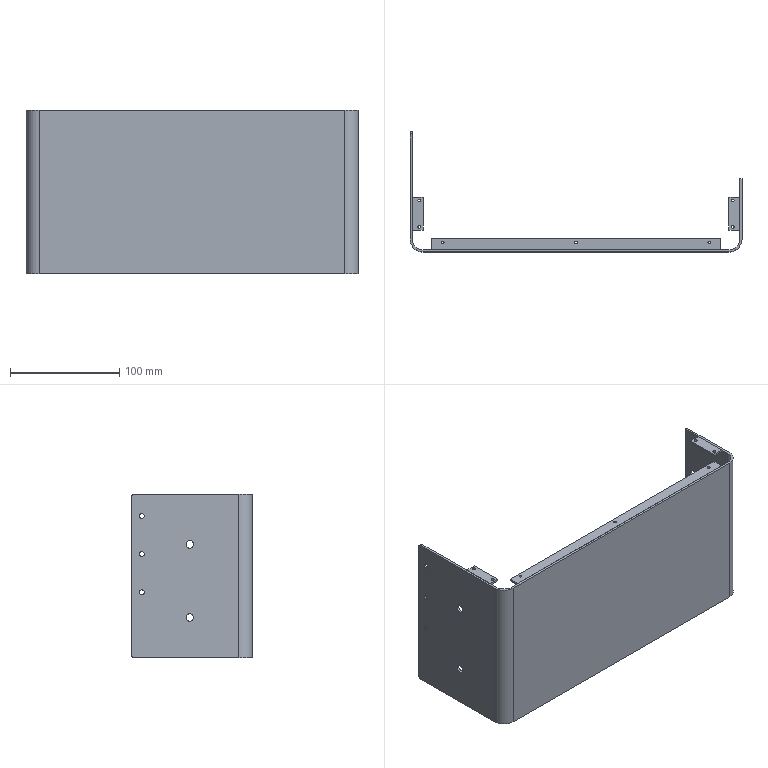Part | STEP file | 11-FG-E02911 | 4 solids | 62 faces | box 304 x 110 x 150 mm | volume 146272 mm3 | cylinder 34 | plane 28 | commonest cylinder face diameters 2.5 x14 7 x8 4.5 x6 4 x2 20 x2 24 x2